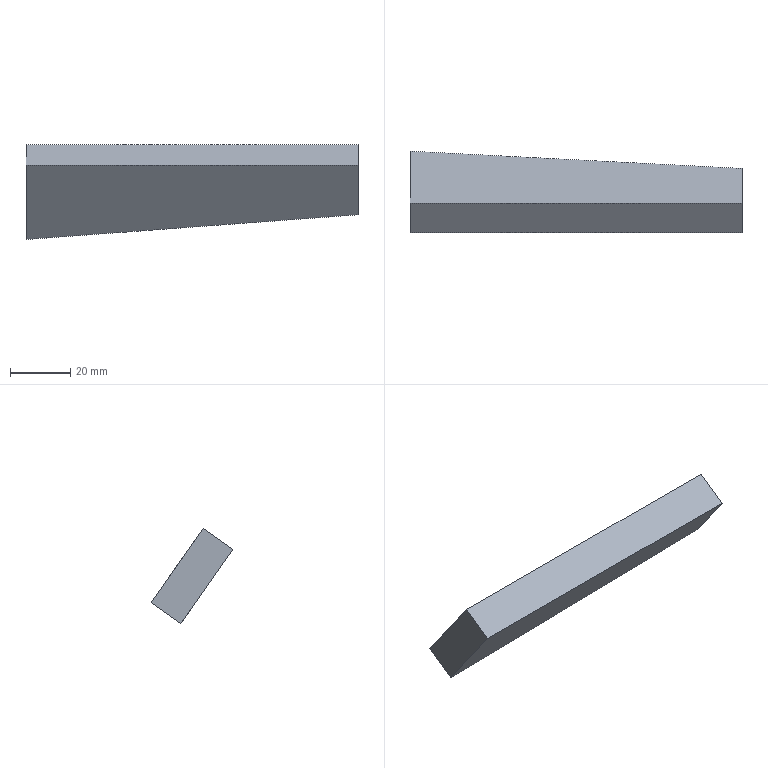Part | STEP file | Positioning_id1806_x_t | 1 solid | 6 faces | box 110 x 27.049 x 31.474 mm | volume 33027 mm3 | plane 6
STEP:
#1=CARTESIAN_POINT('',(0.,0.,0.));
#2=DIRECTION('',(0.,0.,1.));
#3=DIRECTION('',(1.,0.,0.));
#4=AXIS2_PLACEMENT_3D('',#1,#2,#3);
#5=CARTESIAN_POINT('',(-793.002,426.962,345.502));
#6=VERTEX_POINT('',#5);
#7=CARTESIAN_POINT('',(-683.002,421.227,353.693));
#8=VERTEX_POINT('',#7);
#9=CARTESIAN_POINT('',(-793.002,426.962,345.502));
#10=DIRECTION('',(0.9959,-0.05193,0.07416));
#11=VECTOR('',#10,1.);
#12=LINE('',#9,#11);
#13=CARTESIAN_POINT('',(-682.549,421.203,353.727));
#14=DIRECTION('',(0.09054,0.5712,-0.8158));
#15=DIRECTION('',(0.9959,-0.05193,0.07416));
#16=AXIS2_PLACEMENT_3D('',#13,#14,#15);
#17=PLANE('',#16);
#18=CARTESIAN_POINT('',(-110.908,0.));
#19=DIRECTION('',(1.,0.));
#20=VECTOR('',#19,1.);
#21=LINE('',#18,#20);
#22=(GEOMETRIC_REPRESENTATION_CONTEXT(2)PARAMETRIC_REPRESENTATION_CONTEXT()REPRESENTATION_CONTEXT('',''));
#23=DEFINITIONAL_REPRESENTATION('',(#21),#22);
#24=PCURVE('',#17,#23);
#25=CARTESIAN_POINT('',(-731.502,426.951,345.519));
#26=DIRECTION('',(0.,0.8192,0.5736));
#27=DIRECTION('',(1.,0.,0.));
#28=AXIS2_PLACEMENT_3D('',#25,#26,#27);
#29=PLANE('',#28);
#30=CARTESIAN_POINT('',(-61.5,0.02062));
#31=DIRECTION('',(0.9959,-0.09054));
#32=VECTOR('',#31,1.);
#33=LINE('',#30,#32);
#34=(GEOMETRIC_REPRESENTATION_CONTEXT(2)PARAMETRIC_REPRESENTATION_CONTEXT()REPRESENTATION_CONTEXT('',''));
#35=DEFINITIONAL_REPRESENTATION('',(#33),#34);
#36=PCURVE('',#29,#35);
#37=SURFACE_CURVE('',#12,(#24,#36),.PCURVE_S1.);
#38=EDGE_CURVE('',#6,#8,#37,.T.);
#39=ORIENTED_EDGE('',*,*,#38,.T.);
#40=CARTESIAN_POINT('',(-683.002,411.397,346.81));
#41=VERTEX_POINT('',#40);
#42=CARTESIAN_POINT('',(-683.002,421.227,353.693));
#43=DIRECTION('',(0.,-0.8192,-0.5736));
#44=VECTOR('',#43,1.);
#45=LINE('',#42,#44);
#46=CARTESIAN_POINT('',(-0.4545,0.));
#47=DIRECTION('',(0.,1.));
#48=VECTOR('',#47,1.);
#49=LINE('',#46,#48);
#50=(GEOMETRIC_REPRESENTATION_CONTEXT(2)PARAMETRIC_REPRESENTATION_CONTEXT()REPRESENTATION_CONTEXT('',''));
#51=DEFINITIONAL_REPRESENTATION('',(#49),#50);
#52=PCURVE('',#17,#51);
#53=CARTESIAN_POINT('',(-683.002,426.951,345.519));
#54=DIRECTION('',(1.,0.,0.));
#55=DIRECTION('',(0.,-0.8192,-0.5736));
#56=AXIS2_PLACEMENT_3D('',#53,#54,#55);
#57=PLANE('',#56);
#58=CARTESIAN_POINT('',(0.,-9.979));
#59=DIRECTION('',(1.,0.));
#60=VECTOR('',#59,1.);
#61=LINE('',#58,#60);
#62=(GEOMETRIC_REPRESENTATION_CONTEXT(2)PARAMETRIC_REPRESENTATION_CONTEXT()REPRESENTATION_CONTEXT('',''));
#63=DEFINITIONAL_REPRESENTATION('',(#61),#62);
#64=PCURVE('',#57,#63);
#65=SURFACE_CURVE('',#45,(#52,#64),.PCURVE_S1.);
#66=EDGE_CURVE('',#8,#41,#65,.T.);
#67=ORIENTED_EDGE('',*,*,#66,.T.);
#68=CARTESIAN_POINT('',(-793.002,417.133,338.619));
#69=VERTEX_POINT('',#68);
#70=CARTESIAN_POINT('',(-683.002,411.397,346.81));
#71=DIRECTION('',(-0.9959,0.05193,-0.07416));
#72=VECTOR('',#71,1.);
#73=LINE('',#70,#72);
#74=CARTESIAN_POINT('',(-0.4545,12.));
#75=DIRECTION('',(-1.,0.));
#76=VECTOR('',#75,1.);
#77=LINE('',#74,#76);
#78=(GEOMETRIC_REPRESENTATION_CONTEXT(2)PARAMETRIC_REPRESENTATION_CONTEXT()REPRESENTATION_CONTEXT('',''));
#79=DEFINITIONAL_REPRESENTATION('',(#77),#78);
#80=PCURVE('',#17,#79);
#81=CARTESIAN_POINT('',(-731.502,417.121,338.636));
#82=DIRECTION('',(0.,0.8192,0.5736));
#83=DIRECTION('',(1.,0.,0.));
#84=AXIS2_PLACEMENT_3D('',#81,#82,#83);
#85=PLANE('',#84);
#86=CARTESIAN_POINT('',(48.5,-9.979));
#87=DIRECTION('',(-0.9959,0.09054));
#88=VECTOR('',#87,1.);
#89=LINE('',#86,#88);
#90=(GEOMETRIC_REPRESENTATION_CONTEXT(2)PARAMETRIC_REPRESENTATION_CONTEXT()REPRESENTATION_CONTEXT('',''));
#91=DEFINITIONAL_REPRESENTATION('',(#89),#90);
#92=PCURVE('',#85,#91);
#93=SURFACE_CURVE('',#73,(#80,#92),.PCURVE_S1.);
#94=EDGE_CURVE('',#41,#69,#93,.T.);
#95=ORIENTED_EDGE('',*,*,#94,.T.);
#96=CARTESIAN_POINT('',(-793.002,426.962,345.502));
#97=DIRECTION('',(0.,-0.8192,-0.5736));
#98=VECTOR('',#97,1.);
#99=LINE('',#96,#98);
#100=CARTESIAN_POINT('',(-110.908,0.));
#101=DIRECTION('',(0.,1.));
#102=VECTOR('',#101,1.);
#103=LINE('',#100,#102);
#104=(GEOMETRIC_REPRESENTATION_CONTEXT(2)PARAMETRIC_REPRESENTATION_CONTEXT()REPRESENTATION_CONTEXT('',''));
#105=DEFINITIONAL_REPRESENTATION('',(#103),#104);
#106=PCURVE('',#17,#105);
#107=CARTESIAN_POINT('',(-793.002,426.951,345.519));
#108=DIRECTION('',(1.,0.,0.));
#109=DIRECTION('',(0.,-0.8192,-0.5736));
#110=AXIS2_PLACEMENT_3D('',#107,#108,#109);
#111=PLANE('',#110);
#112=CARTESIAN_POINT('',(0.,0.02062));
#113=DIRECTION('',(1.,0.));
#114=VECTOR('',#113,1.);
#115=LINE('',#112,#114);
#116=(GEOMETRIC_REPRESENTATION_CONTEXT(2)PARAMETRIC_REPRESENTATION_CONTEXT()REPRESENTATION_CONTEXT('',''));
#117=DEFINITIONAL_REPRESENTATION('',(#115),#116);
#118=PCURVE('',#111,#117);
#119=SURFACE_CURVE('',#99,(#106,#118),.PCURVE_S1.);
#120=EDGE_CURVE('',#6,#69,#119,.T.);
#121=ORIENTED_EDGE('',*,*,#120,.F.);
#122=EDGE_LOOP('',(#39,#67,#95,#121));
#123=FACE_BOUND('',#122,.T.);
#124=ADVANCED_FACE('',(#123),#17,.T.);
#125=CARTESIAN_POINT('',(-793.002,399.914,363.21));
#126=VERTEX_POINT('',#125);
#127=CARTESIAN_POINT('',(-683.002,399.914,363.21));
#128=VERTEX_POINT('',#127);
#129=CARTESIAN_POINT('',(-793.002,399.914,363.21));
#130=DIRECTION('',(1.,0.,0.));
#131=VECTOR('',#130,1.);
#132=LINE('',#129,#131);
#133=CARTESIAN_POINT('',(-731.502,409.743,370.093));
#134=DIRECTION('',(0.,-0.5736,0.8192));
#135=DIRECTION('',(-1.,0.,0.));
#136=AXIS2_PLACEMENT_3D('',#133,#134,#135);
#137=PLANE('',#136);
#138=CARTESIAN_POINT('',(61.5,12.));
#139=DIRECTION('',(-1.,0.));
#140=VECTOR('',#139,1.);
#141=LINE('',#138,#140);
#142=(GEOMETRIC_REPRESENTATION_CONTEXT(2)PARAMETRIC_REPRESENTATION_CONTEXT()REPRESENTATION_CONTEXT('',''));
#143=DEFINITIONAL_REPRESENTATION('',(#141),#142);
#144=PCURVE('',#137,#143);
#145=CARTESIAN_POINT('',(-61.5,-30.));
#146=DIRECTION('',(1.,0.));
#147=VECTOR('',#146,1.);
#148=LINE('',#145,#147);
#149=(GEOMETRIC_REPRESENTATION_CONTEXT(2)PARAMETRIC_REPRESENTATION_CONTEXT()REPRESENTATION_CONTEXT('',''));
#150=DEFINITIONAL_REPRESENTATION('',(#148),#149);
#151=PCURVE('',#85,#150);
#152=SURFACE_CURVE('',#132,(#144,#151),.PCURVE_S1.);
#153=EDGE_CURVE('',#126,#128,#152,.T.);
#154=ORIENTED_EDGE('',*,*,#153,.T.);
#155=CARTESIAN_POINT('',(-683.002,409.743,370.093));
#156=VERTEX_POINT('',#155);
#157=CARTESIAN_POINT('',(-683.002,409.743,370.093));
#158=DIRECTION('',(0.,-0.8192,-0.5736));
#159=VECTOR('',#158,1.);
#160=LINE('',#157,#159);
#161=CARTESIAN_POINT('',(-48.5,0.));
#162=DIRECTION('',(0.,1.));
#163=VECTOR('',#162,1.);
#164=LINE('',#161,#163);
#165=(GEOMETRIC_REPRESENTATION_CONTEXT(2)PARAMETRIC_REPRESENTATION_CONTEXT()REPRESENTATION_CONTEXT('',''));
#166=DEFINITIONAL_REPRESENTATION('',(#164),#165);
#167=PCURVE('',#137,#166);
#168=CARTESIAN_POINT('',(0.,-30.));
#169=DIRECTION('',(1.,0.));
#170=VECTOR('',#169,1.);
#171=LINE('',#168,#170);
#172=(GEOMETRIC_REPRESENTATION_CONTEXT(2)PARAMETRIC_REPRESENTATION_CONTEXT()REPRESENTATION_CONTEXT('',''));
#173=DEFINITIONAL_REPRESENTATION('',(#171),#172);
#174=PCURVE('',#57,#173);
#175=SURFACE_CURVE('',#160,(#167,#174),.PCURVE_S1.);
#176=EDGE_CURVE('',#156,#128,#175,.T.);
#177=ORIENTED_EDGE('',*,*,#176,.F.);
#178=CARTESIAN_POINT('',(-793.002,409.743,370.093));
#179=VERTEX_POINT('',#178);
#180=CARTESIAN_POINT('',(-793.002,409.743,370.093));
#181=DIRECTION('',(1.,0.,0.));
#182=VECTOR('',#181,1.);
#183=LINE('',#180,#182);
#184=CARTESIAN_POINT('',(61.5,0.));
#185=DIRECTION('',(-1.,0.));
#186=VECTOR('',#185,1.);
#187=LINE('',#184,#186);
#188=(GEOMETRIC_REPRESENTATION_CONTEXT(2)PARAMETRIC_REPRESENTATION_CONTEXT()REPRESENTATION_CONTEXT('',''));
#189=DEFINITIONAL_REPRESENTATION('',(#187),#188);
#190=PCURVE('',#137,#189);
#191=CARTESIAN_POINT('',(-61.5,-30.));
#192=DIRECTION('',(1.,0.));
#193=VECTOR('',#192,1.);
#194=LINE('',#191,#193);
#195=(GEOMETRIC_REPRESENTATION_CONTEXT(2)PARAMETRIC_REPRESENTATION_CONTEXT()REPRESENTATION_CONTEXT('',''));
#196=DEFINITIONAL_REPRESENTATION('',(#194),#195);
#197=PCURVE('',#29,#196);
#198=SURFACE_CURVE('',#183,(#190,#197),.PCURVE_S1.);
#199=EDGE_CURVE('',#179,#156,#198,.T.);
#200=ORIENTED_EDGE('',*,*,#199,.F.);
#201=CARTESIAN_POINT('',(-793.002,409.743,370.093));
#202=DIRECTION('',(0.,-0.8192,-0.5736));
#203=VECTOR('',#202,1.);
#204=LINE('',#201,#203);
#205=CARTESIAN_POINT('',(61.5,0.));
#206=DIRECTION('',(0.,1.));
#207=VECTOR('',#206,1.);
#208=LINE('',#205,#207);
#209=(GEOMETRIC_REPRESENTATION_CONTEXT(2)PARAMETRIC_REPRESENTATION_CONTEXT()REPRESENTATION_CONTEXT('',''));
#210=DEFINITIONAL_REPRESENTATION('',(#208),#209);
#211=PCURVE('',#137,#210);
#212=CARTESIAN_POINT('',(0.,-30.));
#213=DIRECTION('',(1.,0.));
#214=VECTOR('',#213,1.);
#215=LINE('',#212,#214);
#216=(GEOMETRIC_REPRESENTATION_CONTEXT(2)PARAMETRIC_REPRESENTATION_CONTEXT()REPRESENTATION_CONTEXT('',''));
#217=DEFINITIONAL_REPRESENTATION('',(#215),#216);
#218=PCURVE('',#111,#217);
#219=SURFACE_CURVE('',#204,(#211,#218),.PCURVE_S1.);
#220=EDGE_CURVE('',#179,#126,#219,.T.);
#221=ORIENTED_EDGE('',*,*,#220,.T.);
#222=EDGE_LOOP('',(#154,#177,#200,#221));
#223=FACE_BOUND('',#222,.T.);
#224=ADVANCED_FACE('',(#223),#137,.T.);
#225=ORIENTED_EDGE('',*,*,#220,.F.);
#226=CARTESIAN_POINT('',(-793.002,426.962,345.502));
#227=DIRECTION('',(0.,-0.5736,0.8192));
#228=VECTOR('',#227,1.);
#229=LINE('',#226,#228);
#230=CARTESIAN_POINT('',(0.,0.02062));
#231=DIRECTION('',(0.,-1.));
#232=VECTOR('',#231,1.);
#233=LINE('',#230,#232);
#234=(GEOMETRIC_REPRESENTATION_CONTEXT(2)PARAMETRIC_REPRESENTATION_CONTEXT()REPRESENTATION_CONTEXT('',''));
#235=DEFINITIONAL_REPRESENTATION('',(#233),#234);
#236=PCURVE('',#111,#235);
#237=CARTESIAN_POINT('',(-61.5,0.02062));
#238=DIRECTION('',(0.,-1.));
#239=VECTOR('',#238,1.);
#240=LINE('',#237,#239);
#241=(GEOMETRIC_REPRESENTATION_CONTEXT(2)PARAMETRIC_REPRESENTATION_CONTEXT()REPRESENTATION_CONTEXT('',''));
#242=DEFINITIONAL_REPRESENTATION('',(#240),#241);
#243=PCURVE('',#29,#242);
#244=SURFACE_CURVE('',#229,(#236,#243),.PCURVE_S1.);
#245=EDGE_CURVE('',#6,#179,#244,.T.);
#246=ORIENTED_EDGE('',*,*,#245,.F.);
#247=ORIENTED_EDGE('',*,*,#120,.T.);
#248=CARTESIAN_POINT('',(-793.002,417.133,338.619));
#249=DIRECTION('',(0.,-0.5736,0.8192));
#250=VECTOR('',#249,1.);
#251=LINE('',#248,#250);
#252=CARTESIAN_POINT('',(12.,0.02062));
#253=DIRECTION('',(0.,-1.));
#254=VECTOR('',#253,1.);
#255=LINE('',#252,#254);
#256=(GEOMETRIC_REPRESENTATION_CONTEXT(2)PARAMETRIC_REPRESENTATION_CONTEXT()REPRESENTATION_CONTEXT('',''));
#257=DEFINITIONAL_REPRESENTATION('',(#255),#256);
#258=PCURVE('',#111,#257);
#259=CARTESIAN_POINT('',(-61.5,0.02062));
#260=DIRECTION('',(0.,-1.));
#261=VECTOR('',#260,1.);
#262=LINE('',#259,#261);
#263=(GEOMETRIC_REPRESENTATION_CONTEXT(2)PARAMETRIC_REPRESENTATION_CONTEXT()REPRESENTATION_CONTEXT('',''));
#264=DEFINITIONAL_REPRESENTATION('',(#262),#263);
#265=PCURVE('',#85,#264);
#266=SURFACE_CURVE('',#251,(#258,#265),.PCURVE_S1.);
#267=EDGE_CURVE('',#69,#126,#266,.T.);
#268=ORIENTED_EDGE('',*,*,#267,.T.);
#269=EDGE_LOOP('',(#225,#246,#247,#268));
#270=FACE_BOUND('',#269,.T.);
#271=ADVANCED_FACE('',(#270),#111,.F.);
#272=ORIENTED_EDGE('',*,*,#245,.T.);
#273=ORIENTED_EDGE('',*,*,#199,.T.);
#274=CARTESIAN_POINT('',(-683.002,421.227,353.693));
#275=DIRECTION('',(0.,-0.5736,0.8192));
#276=VECTOR('',#275,1.);
#277=LINE('',#274,#276);
#278=CARTESIAN_POINT('',(48.5,-9.979));
#279=DIRECTION('',(0.,-1.));
#280=VECTOR('',#279,1.);
#281=LINE('',#278,#280);
#282=(GEOMETRIC_REPRESENTATION_CONTEXT(2)PARAMETRIC_REPRESENTATION_CONTEXT()REPRESENTATION_CONTEXT('',''));
#283=DEFINITIONAL_REPRESENTATION('',(#281),#282);
#284=PCURVE('',#29,#283);
#285=CARTESIAN_POINT('',(0.,-9.979));
#286=DIRECTION('',(0.,-1.));
#287=VECTOR('',#286,1.);
#288=LINE('',#285,#287);
#289=(GEOMETRIC_REPRESENTATION_CONTEXT(2)PARAMETRIC_REPRESENTATION_CONTEXT()REPRESENTATION_CONTEXT('',''));
#290=DEFINITIONAL_REPRESENTATION('',(#288),#289);
#291=PCURVE('',#57,#290);
#292=SURFACE_CURVE('',#277,(#284,#291),.PCURVE_S1.);
#293=EDGE_CURVE('',#8,#156,#292,.T.);
#294=ORIENTED_EDGE('',*,*,#293,.F.);
#295=ORIENTED_EDGE('',*,*,#38,.F.);
#296=EDGE_LOOP('',(#272,#273,#294,#295));
#297=FACE_BOUND('',#296,.T.);
#298=ADVANCED_FACE('',(#297),#29,.T.);
#299=ORIENTED_EDGE('',*,*,#293,.T.);
#300=ORIENTED_EDGE('',*,*,#176,.T.);
#301=CARTESIAN_POINT('',(-683.002,411.397,346.81));
#302=DIRECTION('',(0.,-0.5736,0.8192));
#303=VECTOR('',#302,1.);
#304=LINE('',#301,#303);
#305=CARTESIAN_POINT('',(12.,-9.979));
#306=DIRECTION('',(0.,-1.));
#307=VECTOR('',#306,1.);
#308=LINE('',#305,#307);
#309=(GEOMETRIC_REPRESENTATION_CONTEXT(2)PARAMETRIC_REPRESENTATION_CONTEXT()REPRESENTATION_CONTEXT('',''));
#310=DEFINITIONAL_REPRESENTATION('',(#308),#309);
#311=PCURVE('',#57,#310);
#312=CARTESIAN_POINT('',(48.5,-9.979));
#313=DIRECTION('',(0.,-1.));
#314=VECTOR('',#313,1.);
#315=LINE('',#312,#314);
#316=(GEOMETRIC_REPRESENTATION_CONTEXT(2)PARAMETRIC_REPRESENTATION_CONTEXT()REPRESENTATION_CONTEXT('',''));
#317=DEFINITIONAL_REPRESENTATION('',(#315),#316);
#318=PCURVE('',#85,#317);
#319=SURFACE_CURVE('',#304,(#311,#318),.PCURVE_S1.);
#320=EDGE_CURVE('',#41,#128,#319,.T.);
#321=ORIENTED_EDGE('',*,*,#320,.F.);
#322=ORIENTED_EDGE('',*,*,#66,.F.);
#323=EDGE_LOOP('',(#299,#300,#321,#322));
#324=FACE_BOUND('',#323,.T.);
#325=ADVANCED_FACE('',(#324),#57,.T.);
#326=ORIENTED_EDGE('',*,*,#320,.T.);
#327=ORIENTED_EDGE('',*,*,#153,.F.);
#328=ORIENTED_EDGE('',*,*,#267,.F.);
#329=ORIENTED_EDGE('',*,*,#94,.F.);
#330=EDGE_LOOP('',(#326,#327,#328,#329));
#331=FACE_BOUND('',#330,.T.);
#332=ADVANCED_FACE('',(#331),#85,.F.);
#333=CLOSED_SHELL('',(#124,#224,#271,#298,#325,#332));
#334=MANIFOLD_SOLID_BREP('',#333);
#335=(LENGTH_UNIT()NAMED_UNIT(*)SI_UNIT(.MILLI.,.METRE.));
#336=UNCERTAINTY_MEASURE_WITH_UNIT(LENGTH_MEASURE(0.0000001),#335,'','');
#337=(NAMED_UNIT(*)PLANE_ANGLE_UNIT()SI_UNIT($,.RADIAN.));
#338=(NAMED_UNIT(*)SI_UNIT($,.STERADIAN.)SOLID_ANGLE_UNIT());
#339=(GEOMETRIC_REPRESENTATION_CONTEXT(3)GLOBAL_UNCERTAINTY_ASSIGNED_CONTEXT((#336))GLOBAL_UNIT_ASSIGNED_CONTEXT((#335,#337,#338))REPRESENTATION_CONTEXT('',''));
#340=ADVANCED_BREP_SHAPE_REPRESENTATION('',(#4,#334),#339);